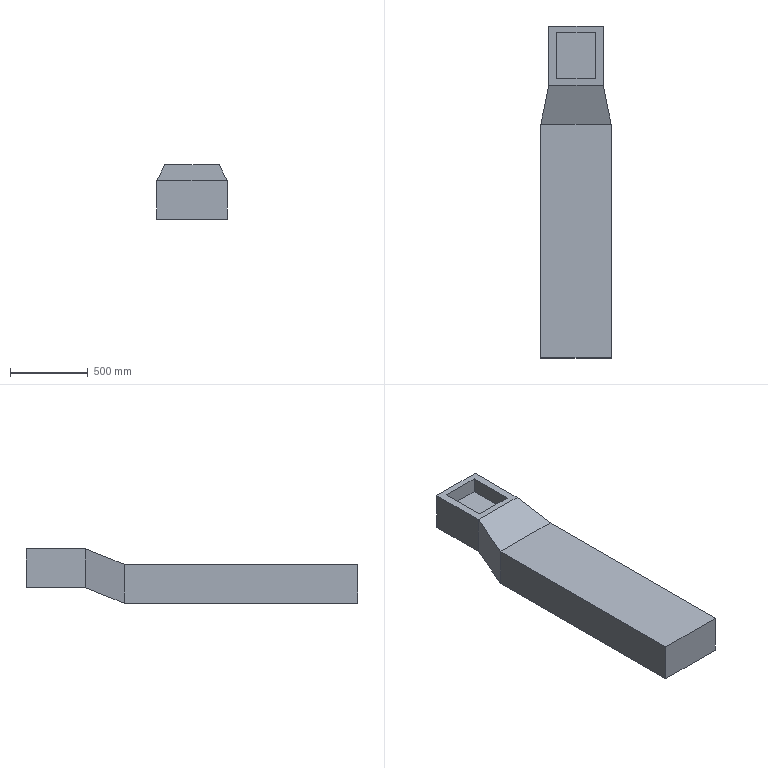Part | SolidWorks | features ICE 2, Extrusion 1 | 1 solid | 19 faces | box 450 x 2130 x 350 mm | volume 219500000 mm3 | plane 19
STEP:
#1=CARTESIAN_POINT('',(175.,-190.,350.));
#2=VERTEX_POINT('',#1);
#3=CARTESIAN_POINT('',(175.,-190.,100.));
#4=VERTEX_POINT('',#3);
#5=CARTESIAN_POINT('',(175.,-190.,350.));
#6=DIRECTION('',(0.,0.,-1.));
#7=VECTOR('',#6,1000.);
#8=LINE('',#5,#7);
#9=EDGE_CURVE('',#2,#4,#8,.T.);
#10=ORIENTED_EDGE('',*,*,#9,.F.);
#11=CARTESIAN_POINT('',(225.,-440.,250.));
#12=VERTEX_POINT('',#11);
#13=CARTESIAN_POINT('',(175.,-190.,350.));
#14=DIRECTION('',(0.1826,-0.9129,-0.3651));
#15=VECTOR('',#14,1000.);
#16=LINE('',#13,#15);
#17=EDGE_CURVE('',#2,#12,#16,.T.);
#18=ORIENTED_EDGE('',*,*,#17,.T.);
#19=CARTESIAN_POINT('',(225.,-440.,0.));
#20=VERTEX_POINT('',#19);
#21=CARTESIAN_POINT('',(225.,-440.,350.));
#22=DIRECTION('',(0.,0.,-1.));
#23=VECTOR('',#22,1000.);
#24=LINE('',#21,#23);
#25=EDGE_CURVE('',#12,#20,#24,.T.);
#26=ORIENTED_EDGE('',*,*,#25,.T.);
#27=CARTESIAN_POINT('',(158.333,-106.667,133.333));
#28=DIRECTION('',(-0.1826,0.9129,0.3651));
#29=VECTOR('',#28,1000.);
#30=LINE('',#27,#29);
#31=EDGE_CURVE('',#20,#4,#30,.T.);
#32=ORIENTED_EDGE('',*,*,#31,.T.);
#33=EDGE_LOOP('',(#10,#18,#26,#32));
#34=FACE_OUTER_BOUND('',#33,.T.);
#35=CARTESIAN_POINT('',(175.,-190.,350.));
#36=DIRECTION('',(-0.9806,-0.1961,0.));
#37=DIRECTION('',(0.1961,-0.9806,0.));
#38=AXIS2_PLACEMENT_3D('',#35,#36,#37);
#39=PLANE('',#38);
#40=ADVANCED_FACE('',(#34),#39,.F.);
#41=ORIENTED_EDGE('',*,*,#9,.T.);
#42=CARTESIAN_POINT('',(175.,190.,100.));
#43=VERTEX_POINT('',#42);
#44=CARTESIAN_POINT('',(175.,190.,100.));
#45=DIRECTION('',(0.,1.,0.));
#46=VECTOR('',#45,1000.);
#47=LINE('',#44,#46);
#48=EDGE_CURVE('',#4,#43,#47,.T.);
#49=ORIENTED_EDGE('',*,*,#48,.T.);
#50=CARTESIAN_POINT('',(175.,190.,350.));
#51=VERTEX_POINT('',#50);
#52=CARTESIAN_POINT('',(175.,190.,350.));
#53=DIRECTION('',(0.,0.,-1.));
#54=VECTOR('',#53,1000.);
#55=LINE('',#52,#54);
#56=EDGE_CURVE('',#51,#43,#55,.T.);
#57=ORIENTED_EDGE('',*,*,#56,.F.);
#58=CARTESIAN_POINT('',(175.,190.,350.));
#59=DIRECTION('',(0.,1.,0.));
#60=VECTOR('',#59,1000.);
#61=LINE('',#58,#60);
#62=EDGE_CURVE('',#2,#51,#61,.T.);
#63=ORIENTED_EDGE('',*,*,#62,.F.);
#64=EDGE_LOOP('',(#41,#49,#57,#63));
#65=FACE_OUTER_BOUND('',#64,.T.);
#66=CARTESIAN_POINT('',(175.,190.,350.));
#67=DIRECTION('',(-1.,0.,0.));
#68=DIRECTION('',(0.,-1.,0.));
#69=AXIS2_PLACEMENT_3D('',#66,#67,#68);
#70=PLANE('',#69);
#71=ADVANCED_FACE('',(#65),#70,.F.);
#72=ORIENTED_EDGE('',*,*,#56,.T.);
#73=CARTESIAN_POINT('',(-175.,190.,100.));
#74=VERTEX_POINT('',#73);
#75=CARTESIAN_POINT('',(225.,190.,100.));
#76=DIRECTION('',(-1.,0.,0.));
#77=VECTOR('',#76,1000.);
#78=LINE('',#75,#77);
#79=EDGE_CURVE('',#43,#74,#78,.T.);
#80=ORIENTED_EDGE('',*,*,#79,.T.);
#81=CARTESIAN_POINT('',(-175.,190.,350.));
#82=VERTEX_POINT('',#81);
#83=CARTESIAN_POINT('',(-175.,190.,350.));
#84=DIRECTION('',(0.,0.,-1.));
#85=VECTOR('',#84,1000.);
#86=LINE('',#83,#85);
#87=EDGE_CURVE('',#82,#74,#86,.T.);
#88=ORIENTED_EDGE('',*,*,#87,.F.);
#89=CARTESIAN_POINT('',(-175.,190.,350.));
#90=DIRECTION('',(-1.,0.,0.));
#91=VECTOR('',#90,1000.);
#92=LINE('',#89,#91);
#93=EDGE_CURVE('',#51,#82,#92,.T.);
#94=ORIENTED_EDGE('',*,*,#93,.F.);
#95=EDGE_LOOP('',(#72,#80,#88,#94));
#96=FACE_OUTER_BOUND('',#95,.T.);
#97=CARTESIAN_POINT('',(-175.,190.,350.));
#98=DIRECTION('',(0.,-1.,0.));
#99=DIRECTION('',(0.,0.,-1.));
#100=AXIS2_PLACEMENT_3D('',#97,#98,#99);
#101=PLANE('',#100);
#102=ADVANCED_FACE('',(#96),#101,.F.);
#103=ORIENTED_EDGE('',*,*,#87,.T.);
#104=CARTESIAN_POINT('',(-175.,-190.,100.));
#105=VERTEX_POINT('',#104);
#106=CARTESIAN_POINT('',(-175.,190.,100.));
#107=DIRECTION('',(0.,-1.,0.));
#108=VECTOR('',#107,1000.);
#109=LINE('',#106,#108);
#110=EDGE_CURVE('',#74,#105,#109,.T.);
#111=ORIENTED_EDGE('',*,*,#110,.T.);
#112=CARTESIAN_POINT('',(-175.,-190.,350.));
#113=VERTEX_POINT('',#112);
#114=CARTESIAN_POINT('',(-175.,-190.,350.));
#115=DIRECTION('',(0.,0.,-1.));
#116=VECTOR('',#115,1000.);
#117=LINE('',#114,#116);
#118=EDGE_CURVE('',#113,#105,#117,.T.);
#119=ORIENTED_EDGE('',*,*,#118,.F.);
#120=CARTESIAN_POINT('',(-175.,190.,350.));
#121=DIRECTION('',(0.,-1.,0.));
#122=VECTOR('',#121,1000.);
#123=LINE('',#120,#122);
#124=EDGE_CURVE('',#82,#113,#123,.T.);
#125=ORIENTED_EDGE('',*,*,#124,.F.);
#126=EDGE_LOOP('',(#103,#111,#119,#125));
#127=FACE_OUTER_BOUND('',#126,.T.);
#128=CARTESIAN_POINT('',(-175.,190.,350.));
#129=DIRECTION('',(1.,0.,0.));
#130=DIRECTION('',(0.,1.,0.));
#131=AXIS2_PLACEMENT_3D('',#128,#129,#130);
#132=PLANE('',#131);
#133=ADVANCED_FACE('',(#127),#132,.F.);
#134=CARTESIAN_POINT('',(-225.,-440.,250.));
#135=VERTEX_POINT('',#134);
#136=CARTESIAN_POINT('',(-225.,-440.,0.));
#137=VERTEX_POINT('',#136);
#138=CARTESIAN_POINT('',(-225.,-440.,350.));
#139=DIRECTION('',(0.,0.,-1.));
#140=VECTOR('',#139,1000.);
#141=LINE('',#138,#140);
#142=EDGE_CURVE('',#135,#137,#141,.T.);
#143=ORIENTED_EDGE('',*,*,#142,.F.);
#144=CARTESIAN_POINT('',(-175.,-190.,350.));
#145=DIRECTION('',(0.1826,0.9129,0.3651));
#146=VECTOR('',#145,1000.);
#147=LINE('',#144,#146);
#148=EDGE_CURVE('',#135,#113,#147,.T.);
#149=ORIENTED_EDGE('',*,*,#148,.T.);
#150=ORIENTED_EDGE('',*,*,#118,.T.);
#151=CARTESIAN_POINT('',(-158.333,-106.667,133.333));
#152=DIRECTION('',(-0.1826,-0.9129,-0.3651));
#153=VECTOR('',#152,1000.);
#154=LINE('',#151,#153);
#155=EDGE_CURVE('',#105,#137,#154,.T.);
#156=ORIENTED_EDGE('',*,*,#155,.T.);
#157=EDGE_LOOP('',(#143,#149,#150,#156));
#158=FACE_OUTER_BOUND('',#157,.T.);
#159=CARTESIAN_POINT('',(-175.,-190.,350.));
#160=DIRECTION('',(0.9806,-0.1961,0.));
#161=DIRECTION('',(0.1961,0.9806,0.));
#162=AXIS2_PLACEMENT_3D('',#159,#160,#161);
#163=PLANE('',#162);
#164=ADVANCED_FACE('',(#158),#163,.F.);
#165=CARTESIAN_POINT('',(-225.,-1940.,250.));
#166=VERTEX_POINT('',#165);
#167=CARTESIAN_POINT('',(-225.,-1940.,0.));
#168=VERTEX_POINT('',#167);
#169=CARTESIAN_POINT('',(-225.,-1940.,350.));
#170=DIRECTION('',(0.,0.,-1.));
#171=VECTOR('',#170,1000.);
#172=LINE('',#169,#171);
#173=EDGE_CURVE('',#166,#168,#172,.T.);
#174=ORIENTED_EDGE('',*,*,#173,.F.);
#175=CARTESIAN_POINT('',(-225.,-440.,250.));
#176=DIRECTION('',(0.,-1.,0.));
#177=VECTOR('',#176,1000.);
#178=LINE('',#175,#177);
#179=EDGE_CURVE('',#135,#166,#178,.T.);
#180=ORIENTED_EDGE('',*,*,#179,.F.);
#181=ORIENTED_EDGE('',*,*,#142,.T.);
#182=CARTESIAN_POINT('',(-225.,-440.,0.));
#183=DIRECTION('',(0.,-1.,0.));
#184=VECTOR('',#183,1000.);
#185=LINE('',#182,#184);
#186=EDGE_CURVE('',#137,#168,#185,.T.);
#187=ORIENTED_EDGE('',*,*,#186,.T.);
#188=EDGE_LOOP('',(#174,#180,#181,#187));
#189=FACE_OUTER_BOUND('',#188,.T.);
#190=CARTESIAN_POINT('',(-225.,-440.,350.));
#191=DIRECTION('',(1.,0.,0.));
#192=DIRECTION('',(0.,1.,0.));
#193=AXIS2_PLACEMENT_3D('',#190,#191,#192);
#194=PLANE('',#193);
#195=ADVANCED_FACE('',(#189),#194,.F.);
#196=CARTESIAN_POINT('',(225.,-1940.,250.));
#197=VERTEX_POINT('',#196);
#198=CARTESIAN_POINT('',(225.,-1940.,0.));
#199=VERTEX_POINT('',#198);
#200=CARTESIAN_POINT('',(225.,-1940.,350.));
#201=DIRECTION('',(0.,0.,-1.));
#202=VECTOR('',#201,1000.);
#203=LINE('',#200,#202);
#204=EDGE_CURVE('',#197,#199,#203,.T.);
#205=ORIENTED_EDGE('',*,*,#204,.F.);
#206=CARTESIAN_POINT('',(225.,-1940.,250.));
#207=DIRECTION('',(-1.,0.,0.));
#208=VECTOR('',#207,1000.);
#209=LINE('',#206,#208);
#210=EDGE_CURVE('',#197,#166,#209,.T.);
#211=ORIENTED_EDGE('',*,*,#210,.T.);
#212=ORIENTED_EDGE('',*,*,#173,.T.);
#213=CARTESIAN_POINT('',(-225.,-1940.,0.));
#214=DIRECTION('',(1.,0.,0.));
#215=VECTOR('',#214,1000.);
#216=LINE('',#213,#215);
#217=EDGE_CURVE('',#168,#199,#216,.T.);
#218=ORIENTED_EDGE('',*,*,#217,.T.);
#219=EDGE_LOOP('',(#205,#211,#212,#218));
#220=FACE_OUTER_BOUND('',#219,.T.);
#221=CARTESIAN_POINT('',(-225.,-1940.,350.));
#222=DIRECTION('',(0.,1.,0.));
#223=DIRECTION('',(0.,0.,1.));
#224=AXIS2_PLACEMENT_3D('',#221,#222,#223);
#225=PLANE('',#224);
#226=ADVANCED_FACE('',(#220),#225,.F.);
#227=ORIENTED_EDGE('',*,*,#25,.F.);
#228=CARTESIAN_POINT('',(225.,-440.,250.));
#229=DIRECTION('',(0.,-1.,0.));
#230=VECTOR('',#229,1000.);
#231=LINE('',#228,#230);
#232=EDGE_CURVE('',#12,#197,#231,.T.);
#233=ORIENTED_EDGE('',*,*,#232,.T.);
#234=ORIENTED_EDGE('',*,*,#204,.T.);
#235=CARTESIAN_POINT('',(225.,-440.,0.));
#236=DIRECTION('',(0.,1.,0.));
#237=VECTOR('',#236,1000.);
#238=LINE('',#235,#237);
#239=EDGE_CURVE('',#199,#20,#238,.T.);
#240=ORIENTED_EDGE('',*,*,#239,.T.);
#241=EDGE_LOOP('',(#227,#233,#234,#240));
#242=FACE_OUTER_BOUND('',#241,.T.);
#243=CARTESIAN_POINT('',(225.,-440.,350.));
#244=DIRECTION('',(-1.,0.,0.));
#245=DIRECTION('',(0.,-1.,0.));
#246=AXIS2_PLACEMENT_3D('',#243,#244,#245);
#247=PLANE('',#246);
#248=ADVANCED_FACE('',(#242),#247,.F.);
#249=CARTESIAN_POINT('',(125.,-150.,350.));
#250=VERTEX_POINT('',#249);
#251=CARTESIAN_POINT('',(125.,150.,350.));
#252=VERTEX_POINT('',#251);
#253=CARTESIAN_POINT('',(125.,150.,350.));
#254=DIRECTION('',(0.,1.,0.));
#255=VECTOR('',#254,1000.);
#256=LINE('',#253,#255);
#257=EDGE_CURVE('',#250,#252,#256,.T.);
#258=ORIENTED_EDGE('',*,*,#257,.F.);
#259=CARTESIAN_POINT('',(-125.,-150.,350.));
#260=VERTEX_POINT('',#259);
#261=CARTESIAN_POINT('',(-125.,-150.,350.));
#262=DIRECTION('',(1.,0.,0.));
#263=VECTOR('',#262,1000.);
#264=LINE('',#261,#263);
#265=EDGE_CURVE('',#260,#250,#264,.T.);
#266=ORIENTED_EDGE('',*,*,#265,.F.);
#267=CARTESIAN_POINT('',(-125.,150.,350.));
#268=VERTEX_POINT('',#267);
#269=CARTESIAN_POINT('',(-125.,150.,350.));
#270=DIRECTION('',(0.,-1.,0.));
#271=VECTOR('',#270,1000.);
#272=LINE('',#269,#271);
#273=EDGE_CURVE('',#268,#260,#272,.T.);
#274=ORIENTED_EDGE('',*,*,#273,.F.);
#275=CARTESIAN_POINT('',(-125.,150.,350.));
#276=DIRECTION('',(-1.,0.,0.));
#277=VECTOR('',#276,1000.);
#278=LINE('',#275,#277);
#279=EDGE_CURVE('',#252,#268,#278,.T.);
#280=ORIENTED_EDGE('',*,*,#279,.F.);
#281=EDGE_LOOP('',(#258,#266,#274,#280));
#282=FACE_BOUND('',#281,.T.);
#283=CARTESIAN_POINT('',(0.,-190.,350.));
#284=DIRECTION('',(-1.,0.,0.));
#285=VECTOR('',#284,1000.);
#286=LINE('',#283,#285);
#287=EDGE_CURVE('',#2,#113,#286,.T.);
#288=ORIENTED_EDGE('',*,*,#287,.F.);
#289=ORIENTED_EDGE('',*,*,#62,.T.);
#290=ORIENTED_EDGE('',*,*,#93,.T.);
#291=ORIENTED_EDGE('',*,*,#124,.T.);
#292=EDGE_LOOP('',(#288,#289,#290,#291));
#293=FACE_OUTER_BOUND('',#292,.T.);
#294=CARTESIAN_POINT('',(0.,0.,350.));
#295=DIRECTION('',(0.,0.,1.));
#296=DIRECTION('',(1.,0.,0.));
#297=AXIS2_PLACEMENT_3D('',#294,#295,#296);
#298=PLANE('',#297);
#299=ADVANCED_FACE('',(#282,#293),#298,.T.);
#300=ORIENTED_EDGE('',*,*,#186,.F.);
#301=CARTESIAN_POINT('',(225.,-440.,0.));
#302=DIRECTION('',(-1.,0.,0.));
#303=VECTOR('',#302,1000.);
#304=LINE('',#301,#303);
#305=EDGE_CURVE('',#20,#137,#304,.T.);
#306=ORIENTED_EDGE('',*,*,#305,.F.);
#307=ORIENTED_EDGE('',*,*,#239,.F.);
#308=ORIENTED_EDGE('',*,*,#217,.F.);
#309=EDGE_LOOP('',(#300,#306,#307,#308));
#310=FACE_OUTER_BOUND('',#309,.T.);
#311=CARTESIAN_POINT('',(0.,0.,0.));
#312=DIRECTION('',(0.,0.,1.));
#313=DIRECTION('',(1.,0.,0.));
#314=AXIS2_PLACEMENT_3D('',#311,#312,#313);
#315=PLANE('',#314);
#316=ADVANCED_FACE('',(#310),#315,.F.);
#317=CARTESIAN_POINT('',(225.,-190.,100.));
#318=DIRECTION('',(-1.,0.,0.));
#319=VECTOR('',#318,1000.);
#320=LINE('',#317,#319);
#321=EDGE_CURVE('',#4,#105,#320,.T.);
#322=ORIENTED_EDGE('',*,*,#321,.T.);
#323=ORIENTED_EDGE('',*,*,#110,.F.);
#324=ORIENTED_EDGE('',*,*,#79,.F.);
#325=ORIENTED_EDGE('',*,*,#48,.F.);
#326=EDGE_LOOP('',(#322,#323,#324,#325));
#327=FACE_OUTER_BOUND('',#326,.T.);
#328=CARTESIAN_POINT('',(225.,-190.,100.));
#329=DIRECTION('',(0.,0.,1.));
#330=DIRECTION('',(0.,-1.,0.));
#331=AXIS2_PLACEMENT_3D('',#328,#329,#330);
#332=PLANE('',#331);
#333=ADVANCED_FACE('',(#327),#332,.F.);
#334=ORIENTED_EDGE('',*,*,#305,.T.);
#335=ORIENTED_EDGE('',*,*,#155,.F.);
#336=ORIENTED_EDGE('',*,*,#321,.F.);
#337=ORIENTED_EDGE('',*,*,#31,.F.);
#338=EDGE_LOOP('',(#334,#335,#336,#337));
#339=FACE_OUTER_BOUND('',#338,.T.);
#340=CARTESIAN_POINT('',(225.,-440.,0.));
#341=DIRECTION('',(0.,-0.3714,0.9285));
#342=DIRECTION('',(0.,-0.9285,-0.3714));
#343=AXIS2_PLACEMENT_3D('',#340,#341,#342);
#344=PLANE('',#343);
#345=ADVANCED_FACE('',(#339),#344,.F.);
#346=ORIENTED_EDGE('',*,*,#287,.T.);
#347=ORIENTED_EDGE('',*,*,#148,.F.);
#348=CARTESIAN_POINT('',(225.,-440.,250.));
#349=DIRECTION('',(-1.,0.,0.));
#350=VECTOR('',#349,1000.);
#351=LINE('',#348,#350);
#352=EDGE_CURVE('',#12,#135,#351,.T.);
#353=ORIENTED_EDGE('',*,*,#352,.F.);
#354=ORIENTED_EDGE('',*,*,#17,.F.);
#355=EDGE_LOOP('',(#346,#347,#353,#354));
#356=FACE_OUTER_BOUND('',#355,.T.);
#357=CARTESIAN_POINT('',(225.,-190.,350.));
#358=DIRECTION('',(0.,0.3714,-0.9285));
#359=DIRECTION('',(0.,0.9285,0.3714));
#360=AXIS2_PLACEMENT_3D('',#357,#358,#359);
#361=PLANE('',#360);
#362=ADVANCED_FACE('',(#356),#361,.F.);
#363=ORIENTED_EDGE('',*,*,#179,.T.);
#364=ORIENTED_EDGE('',*,*,#210,.F.);
#365=ORIENTED_EDGE('',*,*,#232,.F.);
#366=ORIENTED_EDGE('',*,*,#352,.T.);
#367=EDGE_LOOP('',(#363,#364,#365,#366));
#368=FACE_OUTER_BOUND('',#367,.T.);
#369=CARTESIAN_POINT('',(225.,-440.,250.));
#370=DIRECTION('',(0.,0.,-1.));
#371=DIRECTION('',(0.,1.,0.));
#372=AXIS2_PLACEMENT_3D('',#369,#370,#371);
#373=PLANE('',#372);
#374=ADVANCED_FACE('',(#368),#373,.F.);
#375=ORIENTED_EDGE('',*,*,#257,.T.);
#376=CARTESIAN_POINT('',(125.,150.,250.));
#377=VERTEX_POINT('',#376);
#378=CARTESIAN_POINT('',(125.,150.,250.));
#379=DIRECTION('',(0.,0.,1.));
#380=VECTOR('',#379,1000.);
#381=LINE('',#378,#380);
#382=EDGE_CURVE('',#377,#252,#381,.T.);
#383=ORIENTED_EDGE('',*,*,#382,.F.);
#384=CARTESIAN_POINT('',(125.,-150.,250.));
#385=VERTEX_POINT('',#384);
#386=CARTESIAN_POINT('',(125.,150.,250.));
#387=DIRECTION('',(0.,1.,0.));
#388=VECTOR('',#387,1000.);
#389=LINE('',#386,#388);
#390=EDGE_CURVE('',#385,#377,#389,.T.);
#391=ORIENTED_EDGE('',*,*,#390,.F.);
#392=CARTESIAN_POINT('',(125.,-150.,250.));
#393=DIRECTION('',(0.,0.,1.));
#394=VECTOR('',#393,1000.);
#395=LINE('',#392,#394);
#396=EDGE_CURVE('',#385,#250,#395,.T.);
#397=ORIENTED_EDGE('',*,*,#396,.T.);
#398=EDGE_LOOP('',(#375,#383,#391,#397));
#399=FACE_OUTER_BOUND('',#398,.T.);
#400=CARTESIAN_POINT('',(125.,150.,250.));
#401=DIRECTION('',(1.,0.,0.));
#402=DIRECTION('',(0.,1.,0.));
#403=AXIS2_PLACEMENT_3D('',#400,#401,#402);
#404=PLANE('',#403);
#405=ADVANCED_FACE('',(#399),#404,.F.);
#406=ORIENTED_EDGE('',*,*,#265,.T.);
#407=ORIENTED_EDGE('',*,*,#396,.F.);
#408=CARTESIAN_POINT('',(-125.,-150.,250.));
#409=VERTEX_POINT('',#408);
#410=CARTESIAN_POINT('',(-125.,-150.,250.));
#411=DIRECTION('',(1.,0.,0.));
#412=VECTOR('',#411,1000.);
#413=LINE('',#410,#412);
#414=EDGE_CURVE('',#409,#385,#413,.T.);
#415=ORIENTED_EDGE('',*,*,#414,.F.);
#416=CARTESIAN_POINT('',(-125.,-150.,250.));
#417=DIRECTION('',(0.,0.,1.));
#418=VECTOR('',#417,1000.);
#419=LINE('',#416,#418);
#420=EDGE_CURVE('',#409,#260,#419,.T.);
#421=ORIENTED_EDGE('',*,*,#420,.T.);
#422=EDGE_LOOP('',(#406,#407,#415,#421));
#423=FACE_OUTER_BOUND('',#422,.T.);
#424=CARTESIAN_POINT('',(-125.,-150.,250.));
#425=DIRECTION('',(0.,-1.,0.));
#426=DIRECTION('',(0.,0.,-1.));
#427=AXIS2_PLACEMENT_3D('',#424,#425,#426);
#428=PLANE('',#427);
#429=ADVANCED_FACE('',(#423),#428,.F.);
#430=ORIENTED_EDGE('',*,*,#273,.T.);
#431=ORIENTED_EDGE('',*,*,#420,.F.);
#432=CARTESIAN_POINT('',(-125.,150.,250.));
#433=VERTEX_POINT('',#432);
#434=CARTESIAN_POINT('',(-125.,150.,250.));
#435=DIRECTION('',(0.,-1.,0.));
#436=VECTOR('',#435,1000.);
#437=LINE('',#434,#436);
#438=EDGE_CURVE('',#433,#409,#437,.T.);
#439=ORIENTED_EDGE('',*,*,#438,.F.);
#440=CARTESIAN_POINT('',(-125.,150.,250.));
#441=DIRECTION('',(0.,0.,1.));
#442=VECTOR('',#441,1000.);
#443=LINE('',#440,#442);
#444=EDGE_CURVE('',#433,#268,#443,.T.);
#445=ORIENTED_EDGE('',*,*,#444,.T.);
#446=EDGE_LOOP('',(#430,#431,#439,#445));
#447=FACE_OUTER_BOUND('',#446,.T.);
#448=CARTESIAN_POINT('',(-125.,150.,250.));
#449=DIRECTION('',(-1.,0.,0.));
#450=DIRECTION('',(0.,-1.,0.));
#451=AXIS2_PLACEMENT_3D('',#448,#449,#450);
#452=PLANE('',#451);
#453=ADVANCED_FACE('',(#447),#452,.F.);
#454=ORIENTED_EDGE('',*,*,#279,.T.);
#455=ORIENTED_EDGE('',*,*,#444,.F.);
#456=CARTESIAN_POINT('',(-125.,150.,250.));
#457=DIRECTION('',(-1.,0.,0.));
#458=VECTOR('',#457,1000.);
#459=LINE('',#456,#458);
#460=EDGE_CURVE('',#377,#433,#459,.T.);
#461=ORIENTED_EDGE('',*,*,#460,.F.);
#462=ORIENTED_EDGE('',*,*,#382,.T.);
#463=EDGE_LOOP('',(#454,#455,#461,#462));
#464=FACE_OUTER_BOUND('',#463,.T.);
#465=CARTESIAN_POINT('',(-125.,150.,250.));
#466=DIRECTION('',(0.,1.,0.));
#467=DIRECTION('',(0.,0.,1.));
#468=AXIS2_PLACEMENT_3D('',#465,#466,#467);
#469=PLANE('',#468);
#470=ADVANCED_FACE('',(#464),#469,.F.);
#471=ORIENTED_EDGE('',*,*,#390,.T.);
#472=ORIENTED_EDGE('',*,*,#460,.T.);
#473=ORIENTED_EDGE('',*,*,#438,.T.);
#474=ORIENTED_EDGE('',*,*,#414,.T.);
#475=EDGE_LOOP('',(#471,#472,#473,#474));
#476=FACE_OUTER_BOUND('',#475,.T.);
#477=CARTESIAN_POINT('',(0.,0.,250.));
#478=DIRECTION('',(0.,0.,1.));
#479=DIRECTION('',(1.,0.,0.));
#480=AXIS2_PLACEMENT_3D('',#477,#478,#479);
#481=PLANE('',#480);
#482=ADVANCED_FACE('',(#476),#481,.T.);
#483=CLOSED_SHELL('',(#40,#71,#102,#133,#164,#195,#226,#248,#299,#316,#333,#345,#362,#374,#405,#429,#453,#470,#482));
#484=MANIFOLD_SOLID_BREP('',#483);
#485=CARTESIAN_POINT('',(0.,0.,0.));
#486=DIRECTION('',(0.,0.,1.));
#487=DIRECTION('',(1.,0.,0.));
#488=AXIS2_PLACEMENT_3D('',#485,#486,#487);
#489=(LENGTH_UNIT()NAMED_UNIT(*)SI_UNIT(.MILLI.,.METRE.));
#490=UNCERTAINTY_MEASURE_WITH_UNIT(LENGTH_MEASURE(0.00001),#489,'','');
#491=(NAMED_UNIT(*)PLANE_ANGLE_UNIT()SI_UNIT($,.RADIAN.));
#492=(NAMED_UNIT(*)SI_UNIT($,.STERADIAN.)SOLID_ANGLE_UNIT());
#493=(GEOMETRIC_REPRESENTATION_CONTEXT(3)GLOBAL_UNCERTAINTY_ASSIGNED_CONTEXT((#490))GLOBAL_UNIT_ASSIGNED_CONTEXT((#489,#491,#492))REPRESENTATION_CONTEXT('',''));
#494=ADVANCED_BREP_SHAPE_REPRESENTATION('',(#484,#488),#493);